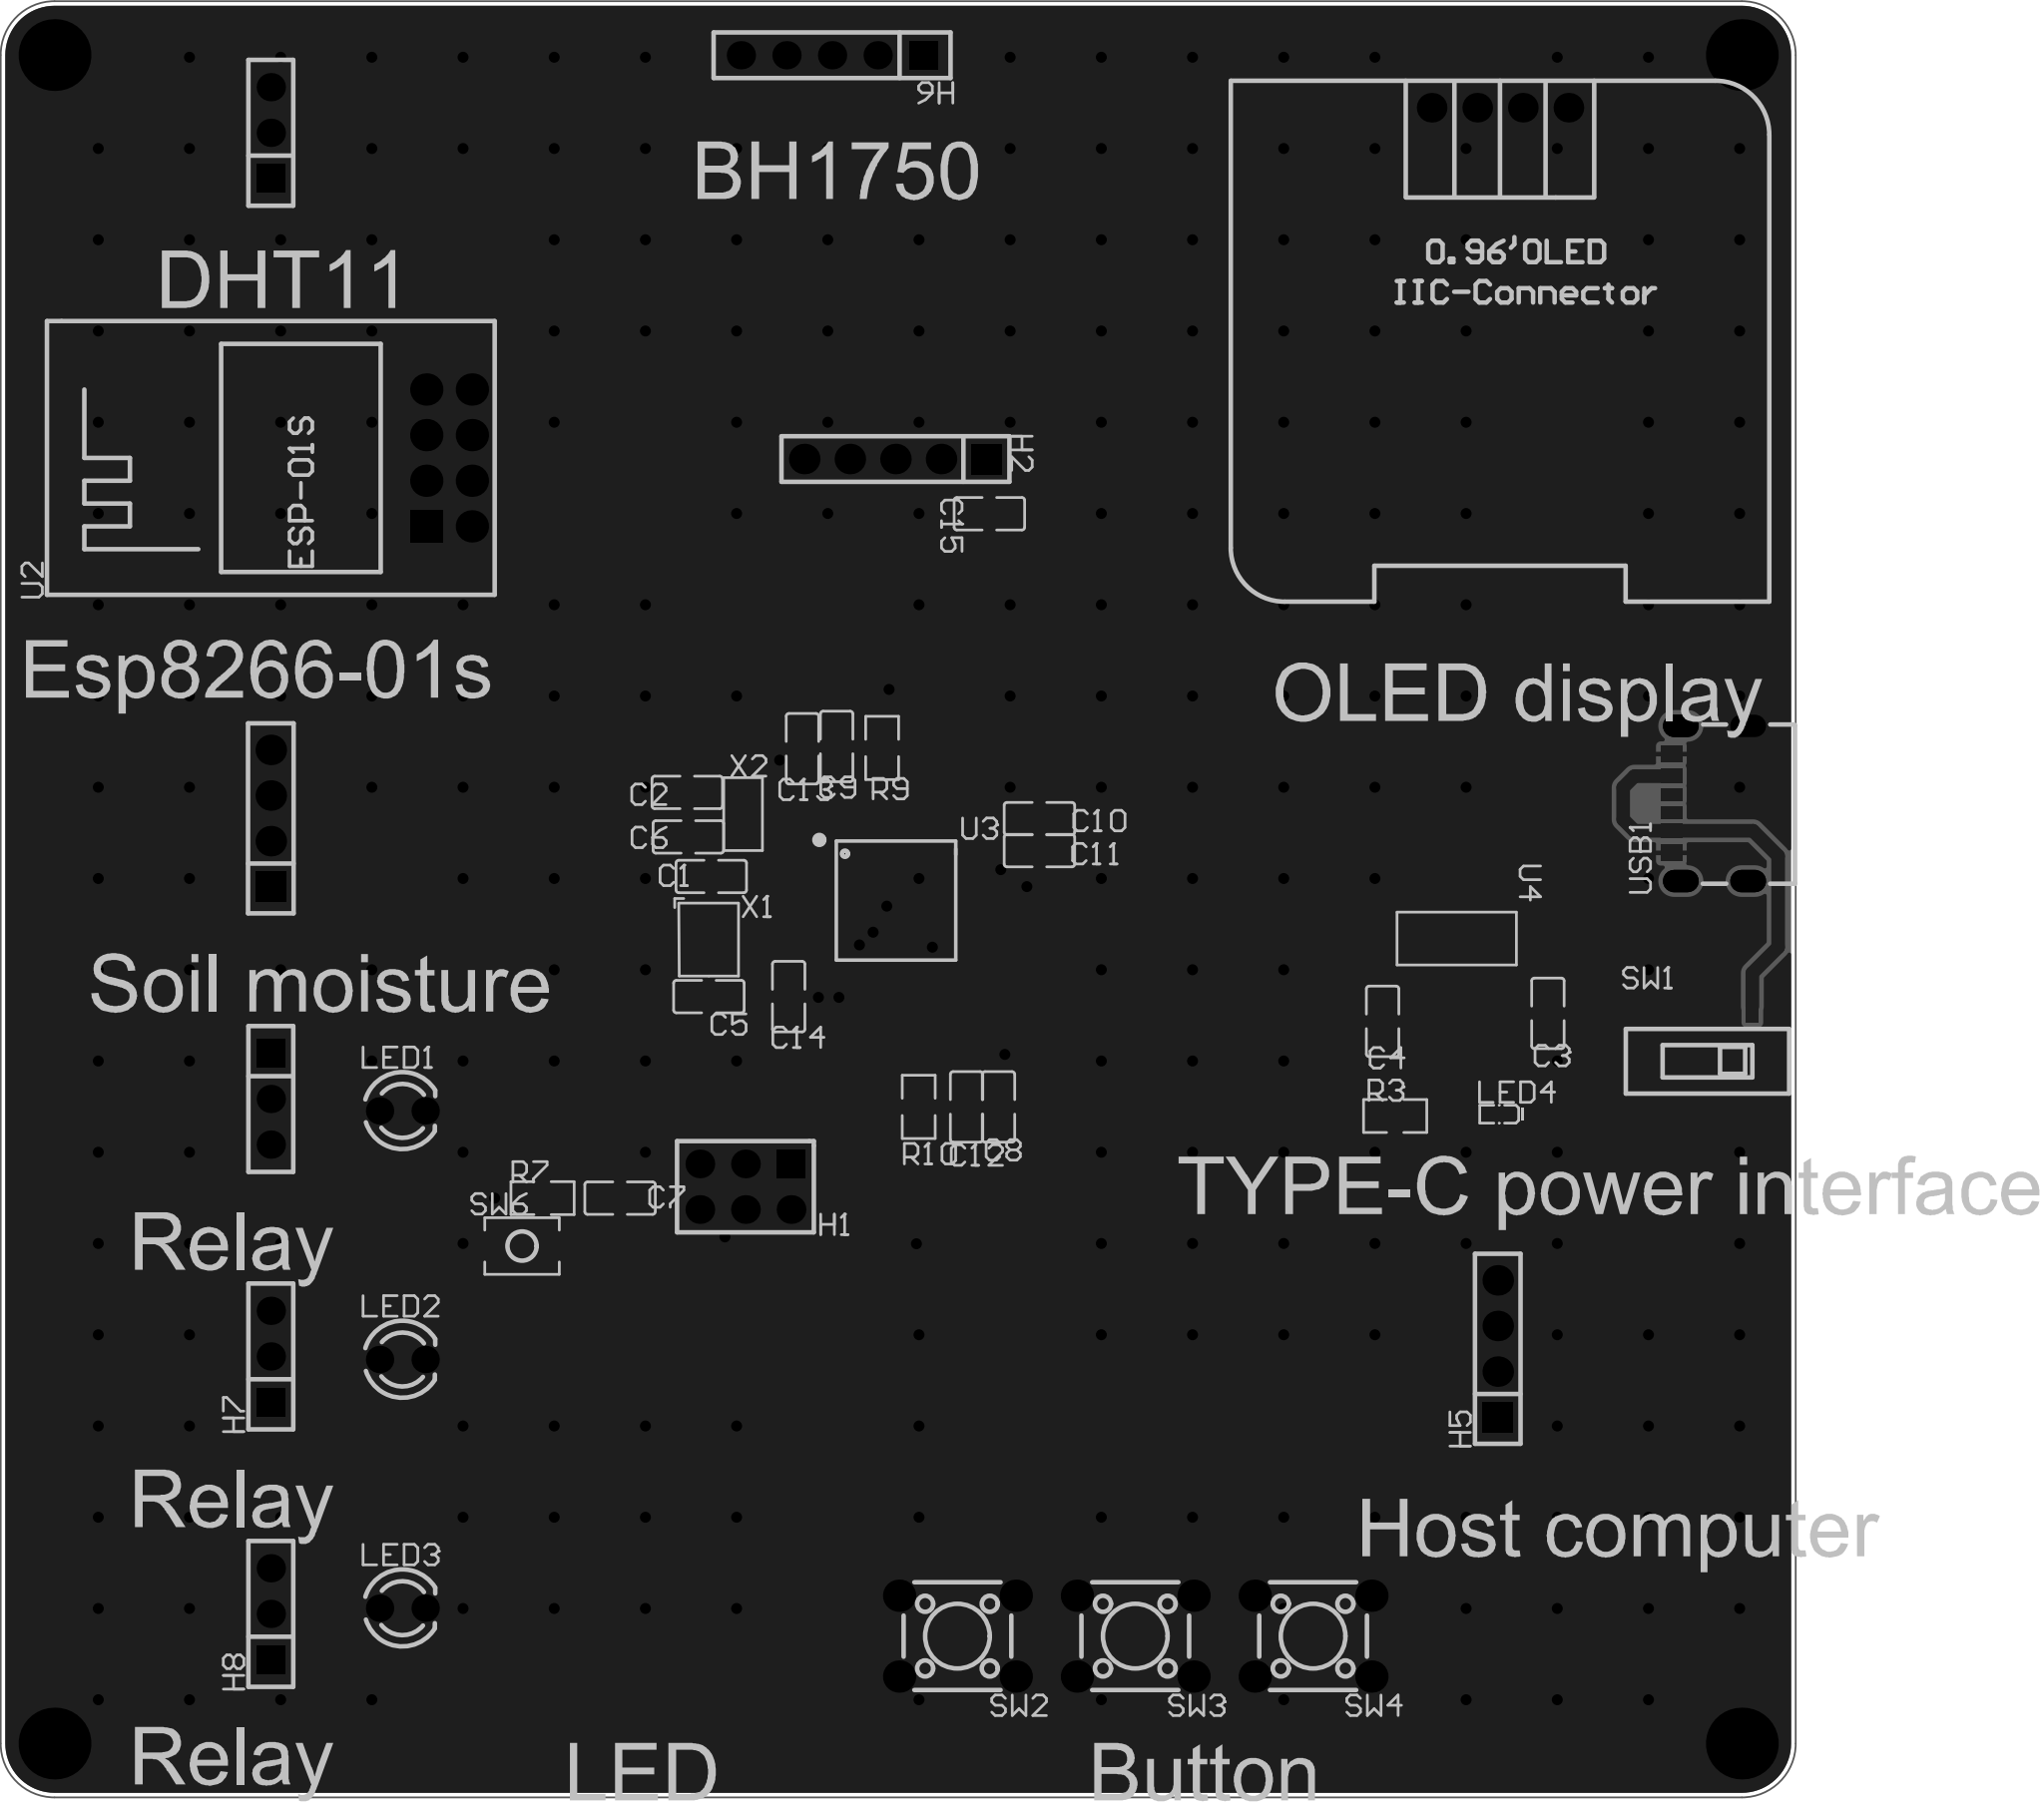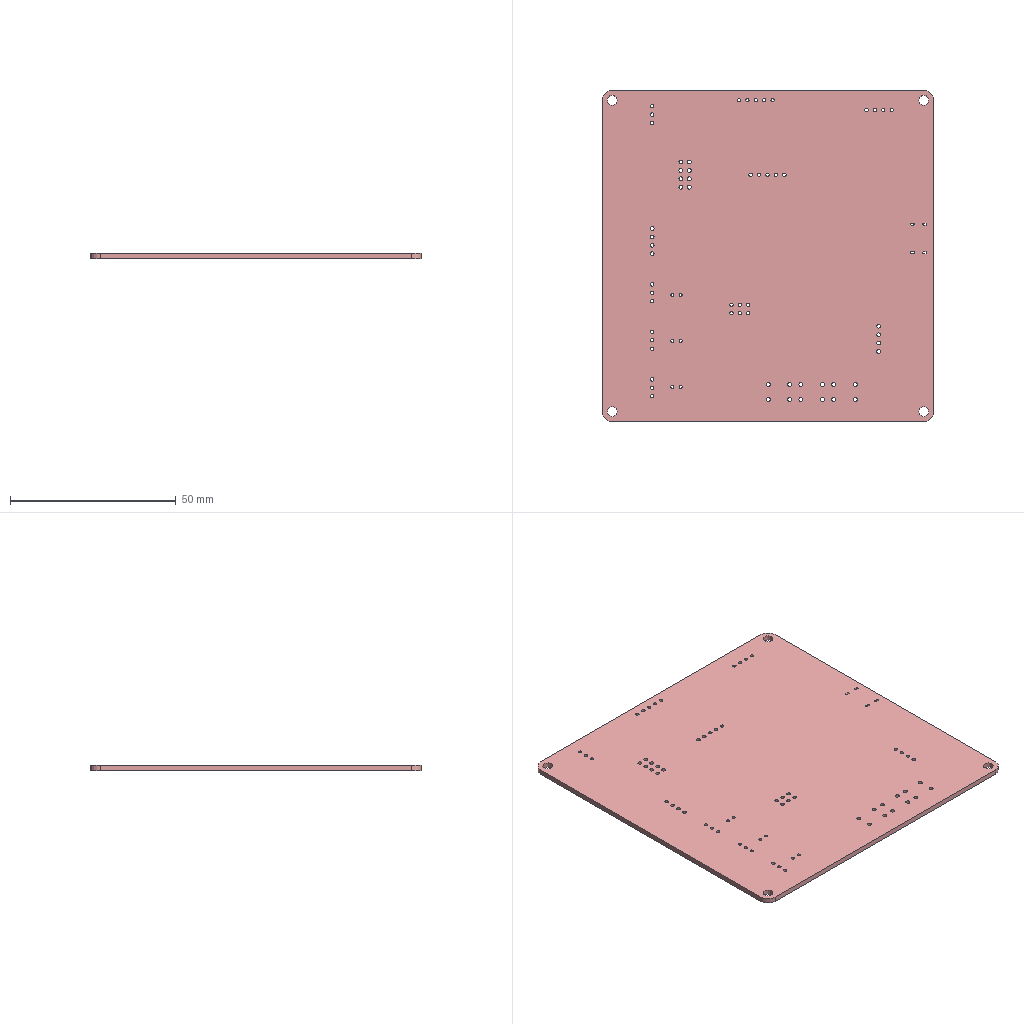Circuit board layout | Altium Designer | box 100 x 100 x 1.6 mm
Layer stack:
# Altium Designer layer stack of  (unit mm; dielectric type: 0 none, 1 core, 2 prepreg, 3 surface material)
index,name,kind,layer,copper_thickness_mm,dielectric_type,dielectric_thickness_mm,dielectric_material,dielectric_constant
0,Top Paste Mask Layer,other,,,,,,
1,Top Silkscreen Layer,other,,,,,,
2,Top Solder Mask Layer,dielectric,,,3,0.01,,3.3
3,Top Layer,copper,Top Layer,0.035,,,,
4,Dielectric1,dielectric,,,3,1.51,FR4,4.5
5,Bottom Layer,copper,Bottom Layer,0.035,,,,
6,Bottom Solder Mask Layer,dielectric,,,3,0.01,,3.3
7,Bottom Silkscreen Layer,other,,,,,,
8,Bottom Paste Mask Layer,other,,,,,,
# drill layer pairs: low layer,high layer
drill_pair,Top Layer,Bottom Layer
Part placement:
Designator,Comment,Layer,Footprint,Center-X(mm),Center-Y(mm),Rotation
OLED1,,TopLayer,0.96OLED_4P,174.879,175.006,0
SW2,,TopLayer,SW-TH_4P-L6.0-W6.0-P4.50-LS6.5,144.653,89.916,180
SW3,,TopLayer,SW-TH_4P-L6.0-W6.0-P4.50-LS6.5,154.559,89.916,180
SW4,,TopLayer,SW-TH_4P-L6.0-W6.0-P4.50-LS6.5,164.465,89.916,180
H12,,TopLayer,HDR-TH_3P-P2.54-V-F,106.401,119.82,270
H3,,TopLayer,HDR-TH_3P-P2.54-V-F,106.401,173.609,90
H4,,TopLayer,HDR-TH_4P-P2.54-V-F,106.401,135.444,90
H5,,TopLayer,HDR-TH_4P-P2.54-V-F,174.752,105.913,90
H6,,TopLayer,HDR-TH_5P-P2.54-V-F,137.668,177.927,180
H7,,TopLayer,HDR-TH_3P-P2.54-V-F,106.401,105.487,90
H8,,TopLayer,HDR-TH_3P-P2.54-V-F,106.401,91.153,90
LED1,,TopLayer,LED_TH-3mm,113.73,119.158,0
LED2,,TopLayer,LED_TH-3mm,113.73,105.315,0
LED3,,TopLayer,LED_TH-3mm,113.73,91.472,0
U2,ESP-01S,TopLayer,WIFIM-TH_ESP-01S,116.332,155.509,90
USB1,,TopLayer,USB__TYPE-C-6P,186.563,136.271,90
U3,STM32F103C8T6,TopLayer,LQFP-48_L7.0-W7.0-P0.50-LS9.0-BL,141.218,130.854,270
H1,,TopLayer,HDR-TH_6P-P2.54-V-R2-C3-S2.54_A2541WV-2X3P,132.842,114.935,180
X1,8MHz,TopLayer,OSC-SMD_4P-L3.2-W2.5-BL,130.804,128.695,270
X2,32.768kHz,TopLayer,CRYSTAL-SMD_L3.2-W1.5-1,132.709,135.68,90
H2,PZ254V-11-05P,TopLayer,HDR-TH_5P-P2.54-V-M,141.198,155.447,180
LED4,,TopLayer,LED_0402,174.832,118.975,180
SW1,SS-3235S-L1,TopLayer,SW-SMD_SS-3235S-LX,186.436,121.92,0
SW6,,TopLayer,Key_SMD_3x4x2,120.396,111.633,0
U4,AMS1117-3.3,TopLayer,SOT-223-3_L6.5-W3.4-P2.30-LS7.0-BR,172.466,128.651,270
C1,18pF,TopLayer,C0805,130.937,132.207,0
C2,10pF,TopLayer,C0805,129.599,136.888,0
C3,1uF,TopLayer,C0805,177.546,124.587,90
C4,1uF,TopLayer,C0805,168.337,124.141,270
C5,18pF,TopLayer,C0805,130.804,125.52,180
C6,10pF,TopLayer,C0805,129.661,134.41,0
C7,1uF,TopLayer,C0805,125.857,114.3,0
C8,4.7uF,TopLayer,C0805,146.939,119.38,90
C9,100nF,TopLayer,C0805,137.922,139.446,90
C10,100nF,TopLayer,C0805,149.219,135.426,0
C11,100nF,TopLayer,C0805,149.219,133.648,180
C12,100nF,TopLayer,C0805,145.161,119.38,90
C13,100nF,TopLayer,C0805,136.017,139.319,270
C14,100nF,TopLayer,C0805,135.249,125.52,90
C15,100nF,TopLayer,C0805,146.431,152.4,0
R3,1kΩ,TopLayer,R0805,169.037,118.872,0
R7,10kΩ,TopLayer,R0805,121.539,114.3,180
R9,10kΩ,TopLayer,R0805,140.456,139.363,90
R10,10kΩ,TopLayer,R0805,142.494,119.38,90
Pad and via stacks:
# Altium Designer via and pad stacks of  (unit mm). Each distinct definition once, with the count of objects using it.
# via: kind,start_layer,end_layer,hole_mm,diameter_mm,mode(0 simple;1 top-mid-bottom;2 full stack),diameter_per_layer,count,example_net
# pad: kind,layer,hole_mm,hole_type(0 round;1 square;2 slot),plating,top_size,top_shape(1 round;2 rect;3 octagon;9 rounded rect),mid_size,bottom_size,mode,footprint,size_per_layer,count,example
pad,Multi-Layer,3,0,plated,4x4,1,4x4,4x4,0,,,4,1
pad,Multi-Layer,1,0,plated,1.65x1.65,1,1.65x1.65,1.65x1.65,0,0.96OLED_4P,,4,OLED1.4
pad,Multi-Layer,1.2,0,plated,1.8x1.8,1,1.8x1.8,1.8x1.8,0,SW-TH_4P-L6.0-W6.0-P4.50-LS6.5,,12,SW2.1
pad,Multi-Layer,1.02,0,plated,1.575x1.575,1,1.575x1.575,1.575x1.575,0,HDR-TH_3P-P2.54-V-F,,8,H12.3
pad,Multi-Layer,1.02,0,plated,1.575x1.575,2,1.575x1.575,1.575x1.575,0,HDR-TH_3P-P2.54-V-F,,4,H12.1
pad,Multi-Layer,1.1,0,plated,1.7x1.7,2,1.7x1.7,1.7x1.7,0,HDR-TH_4P-P2.54-V-F,,2,H4.1
pad,Multi-Layer,1.1,0,plated,1.7x1.7,1,1.7x1.7,1.7x1.7,0,HDR-TH_4P-P2.54-V-F,,6,H4.2
pad,Multi-Layer,1.02,0,plated,1.575x1.575,1,1.575x1.575,1.575x1.575,0,HDR-TH_5P-P2.54-V-F,,4,H6.5
pad,Multi-Layer,1.02,0,plated,1.575x1.575,2,1.575x1.575,1.575x1.575,0,HDR-TH_5P-P2.54-V-F,,1,H6.1
pad,Multi-Layer,0.9144,0,plated,1.524x1.524,1,1.524x1.524,1.524x1.524,0,LED_TH-3mm,,6,LED1.1
pad,Multi-Layer,1.2,0,plated,1.8x1.8,2,1.8x1.8,1.8x1.8,0,WIFIM-TH_ESP-01S,,1,U2.1
pad,Multi-Layer,1.2,0,plated,1.8x1.8,1,1.8x1.8,1.8x1.8,0,WIFIM-TH_ESP-01S,,7,U2.2
pad,Multi-Layer,0.6,2,plated,1.25x2,1,1.25x2,1.25x2,0,USB_ TYPE-C-6P,,4,USB1.8
pad,Multi-Layer,1.05,0,plated,1.6x1.6,2,1.6x1.6,1.6x1.6,0,HDR-TH_6P-P2.54-V-R2-C3-S2.54_A2541WV-2X3P,,1,H1.1
pad,Multi-Layer,1.05,0,plated,1.6x1.6,1,1.6x1.6,1.6x1.6,0,HDR-TH_6P-P2.54-V-R2-C3-S2.54_A2541WV-2X3P,,5,H1.2
pad,Multi-Layer,1.1,0,plated,1.7x1.7,2,1.7x1.7,1.7x1.7,0,HDR-TH_5P-P2.54-V-M,,1,H2.1
pad,Multi-Layer,1.1,0,plated,1.7x1.7,1,1.7x1.7,1.7x1.7,0,HDR-TH_5P-P2.54-V-M,,4,H2.2
pad,Top Layer,0,0,plated,0.7x1.2,2,0.7x1.2,0.7x1.2,0,USB_ TYPE-C-6P,,2,USB1.A5
pad,Top Layer,0,0,plated,0.8x1.2,2,0.8x1.2,0.8x1.2,0,USB_ TYPE-C-6P,,2,USB1.B9
pad,Top Layer,0,0,plated,0.9x1.2,2,0.9x1.2,0.9x1.2,0,USB_ TYPE-C-6P,,2,USB1.B12
pad,Top Layer,0,0,plated,0.27x1.5,1,0.27x1.5,0.27x1.5,0,LQFP-48_L7.0-W7.0-P0.50-LS9.0-BL,,24,U3.1
pad,Top Layer,0,0,plated,1.5x0.27,1,1.5x0.27,1.5x0.27,0,LQFP-48_L7.0-W7.0-P0.50-LS9.0-BL,,24,U3.13
pad,Top Layer,0,0,plated,1.4x1.2,2,1.4x1.2,1.4x1.2,0,OSC-SMD_4P-L3.2-W2.5-BL,,4,X1.1
pad,Top Layer,0,0,plated,1.05x1.7,2,1.05x1.7,1.05x1.7,0,CRYSTAL-SMD_L3.2-W1.5-1,,2,X2.2
pad,Top Layer,0,0,plated,0.6375x0.541,2,0.6375x0.541,0.6375x0.541,0,LED_0402,,2,LED4.2
pad,Top Layer,0,0,plated,0.7x1.8,2,0.7x1.8,0.7x1.8,0,SW-SMD_SS-3235S-LX,,6,SW1.1
pad,Top Layer,0,0,plated,1.53x1.36,2,1.53x1.36,1.53x1.36,0,Key_SMD_3x4x2,,2,SW6.1
pad,Top Layer,0,0,plated,2.5x1.1,2,2.5x1.1,2.5x1.1,0,SOT-223-3_L6.5-W3.4-P2.30-LS7.0-BR,,3,U4.1
pad,Top Layer,0,0,plated,2.34x3.6,2,2.34x3.6,2.34x3.6,0,SOT-223-3_L6.5-W3.4-P2.30-LS7.0-BR,,1,U4.4
pad,Top Layer,0,0,plated,1.41x1.35,2,1.41x1.35,1.41x1.35,0,C0805,,30,C1.2
pad,Top Layer,0,0,plated,1.133x1.377,2,1.133x1.377,1.133x1.377,0,R0805,,8,R3.2
via,Top Layer,Bottom Layer,0.3048,0.61,0,,265,PA0
Copper pours:
name,layer,net,type(0 solid;1 hatched;2 none)
Bottom Layer-GND,Bottom Layer,GND,0
Top Layer-GND,Top Layer,GND,0
Design rules, without the lines most boards share:
# Altium Designer design rules of  (exported by Altium Designer, unit mm)
# columns: name | kind | enabled | priority | scope1 | scope2 | descriptor | typed fields (field=value)
Copper_copperRegion_copperThickness1oz | 0 | disabled | 4 | All | All | Clearance Constraint (Gap=5.984mil) (Disabled)(All),(All) | gap=0.152
Copper_copperRegion_copperThickness1oz_1 | 63 | disabled | 4 | All | All | Board Clearance Constraint (Gap=0mil) (Disabled)(All) |
Copper_copperRegion_Copper_copperRegion | 0 | disabled | 5 | All | All | Clearance Constraint (Gap=5.984mil) (Disabled)(All),(All) | gap=0.152
Copper_copperRegion_Copper_copperRegion_1 | 63 | disabled | 5 | All | All | Board Clearance Constraint (Gap=0mil) (Disabled)(All) |
copperThickness1oz | 0 | enabled | 6 | All | All | Clearance Constraint (Gap=5.984mil) (All),(All) | gap=0.152
copperThickness1oz_1 | 63 | enabled | 6 | All | All | Board Clearance Constraint (Gap=0mil) (All) |
copperRegion_copperThickness1oz | 20 | disabled | 1 | All | All | Polygon Connect Rule(Relief Connect )(Conductor Width=10mil) (Relief Angle=90 Angle) (Entries=4) (Air Gap Width=10mil) (Disabled)(All),(All) | connect_style(0=relief,1=direct,2=none)=0 relief_conductor_width=0.254 relief_entries=4
copperRegion_Copper_copperRegion | 20 | disabled | 2 | All | All | Polygon Connect Rule(Relief Connect )(Conductor Width=10mil) (Relief Angle=90 Angle) (Entries=4) (Air Gap Width=10mil) (Disabled)(All),(All) | connect_style(0=relief,1=direct,2=none)=0 relief_conductor_width=0.254 relief_entries=4
copperRegion | 20 | enabled | 3 | All | All | Polygon Connect Rule(Relief Connect )(Conductor Width=10mil) (Relief Angle=90 Angle) (Entries=4) (Air Gap Width=10mil) (All),(All) | connect_style(0=relief,1=direct,2=none)=0 relief_conductor_width=0.254 relief_entries=4